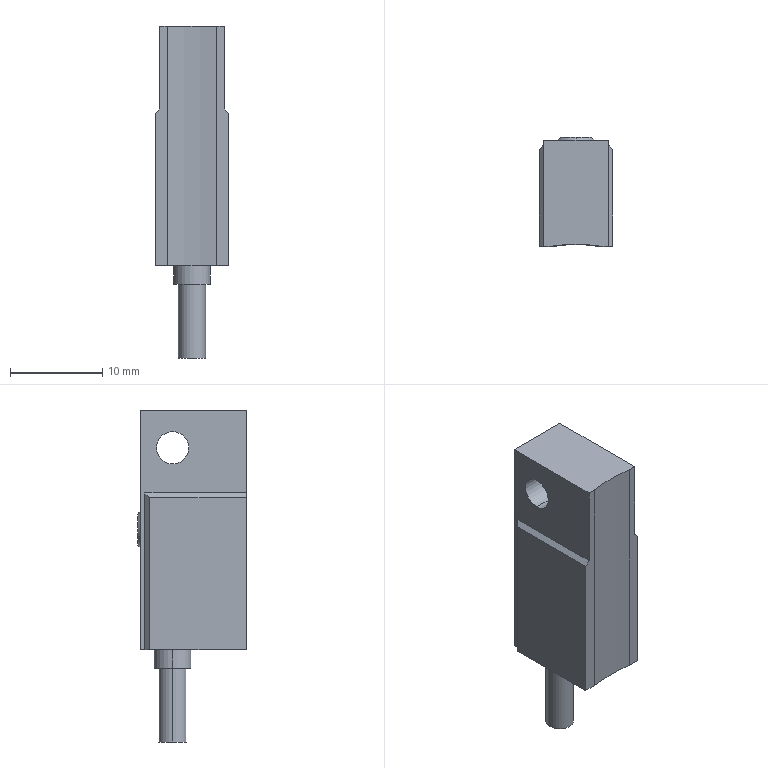Part | STEP file | QA-HI_SB-CS-130_3 | 1 solid | 30 faces | box 8 x 11.8 x 36 mm | volume 2270 mm3 | plane 21 | cylinder 7 | cone 2 | commonest cylinder face diameters 3 x2 3.5 x2 4 x2 36.4 x1